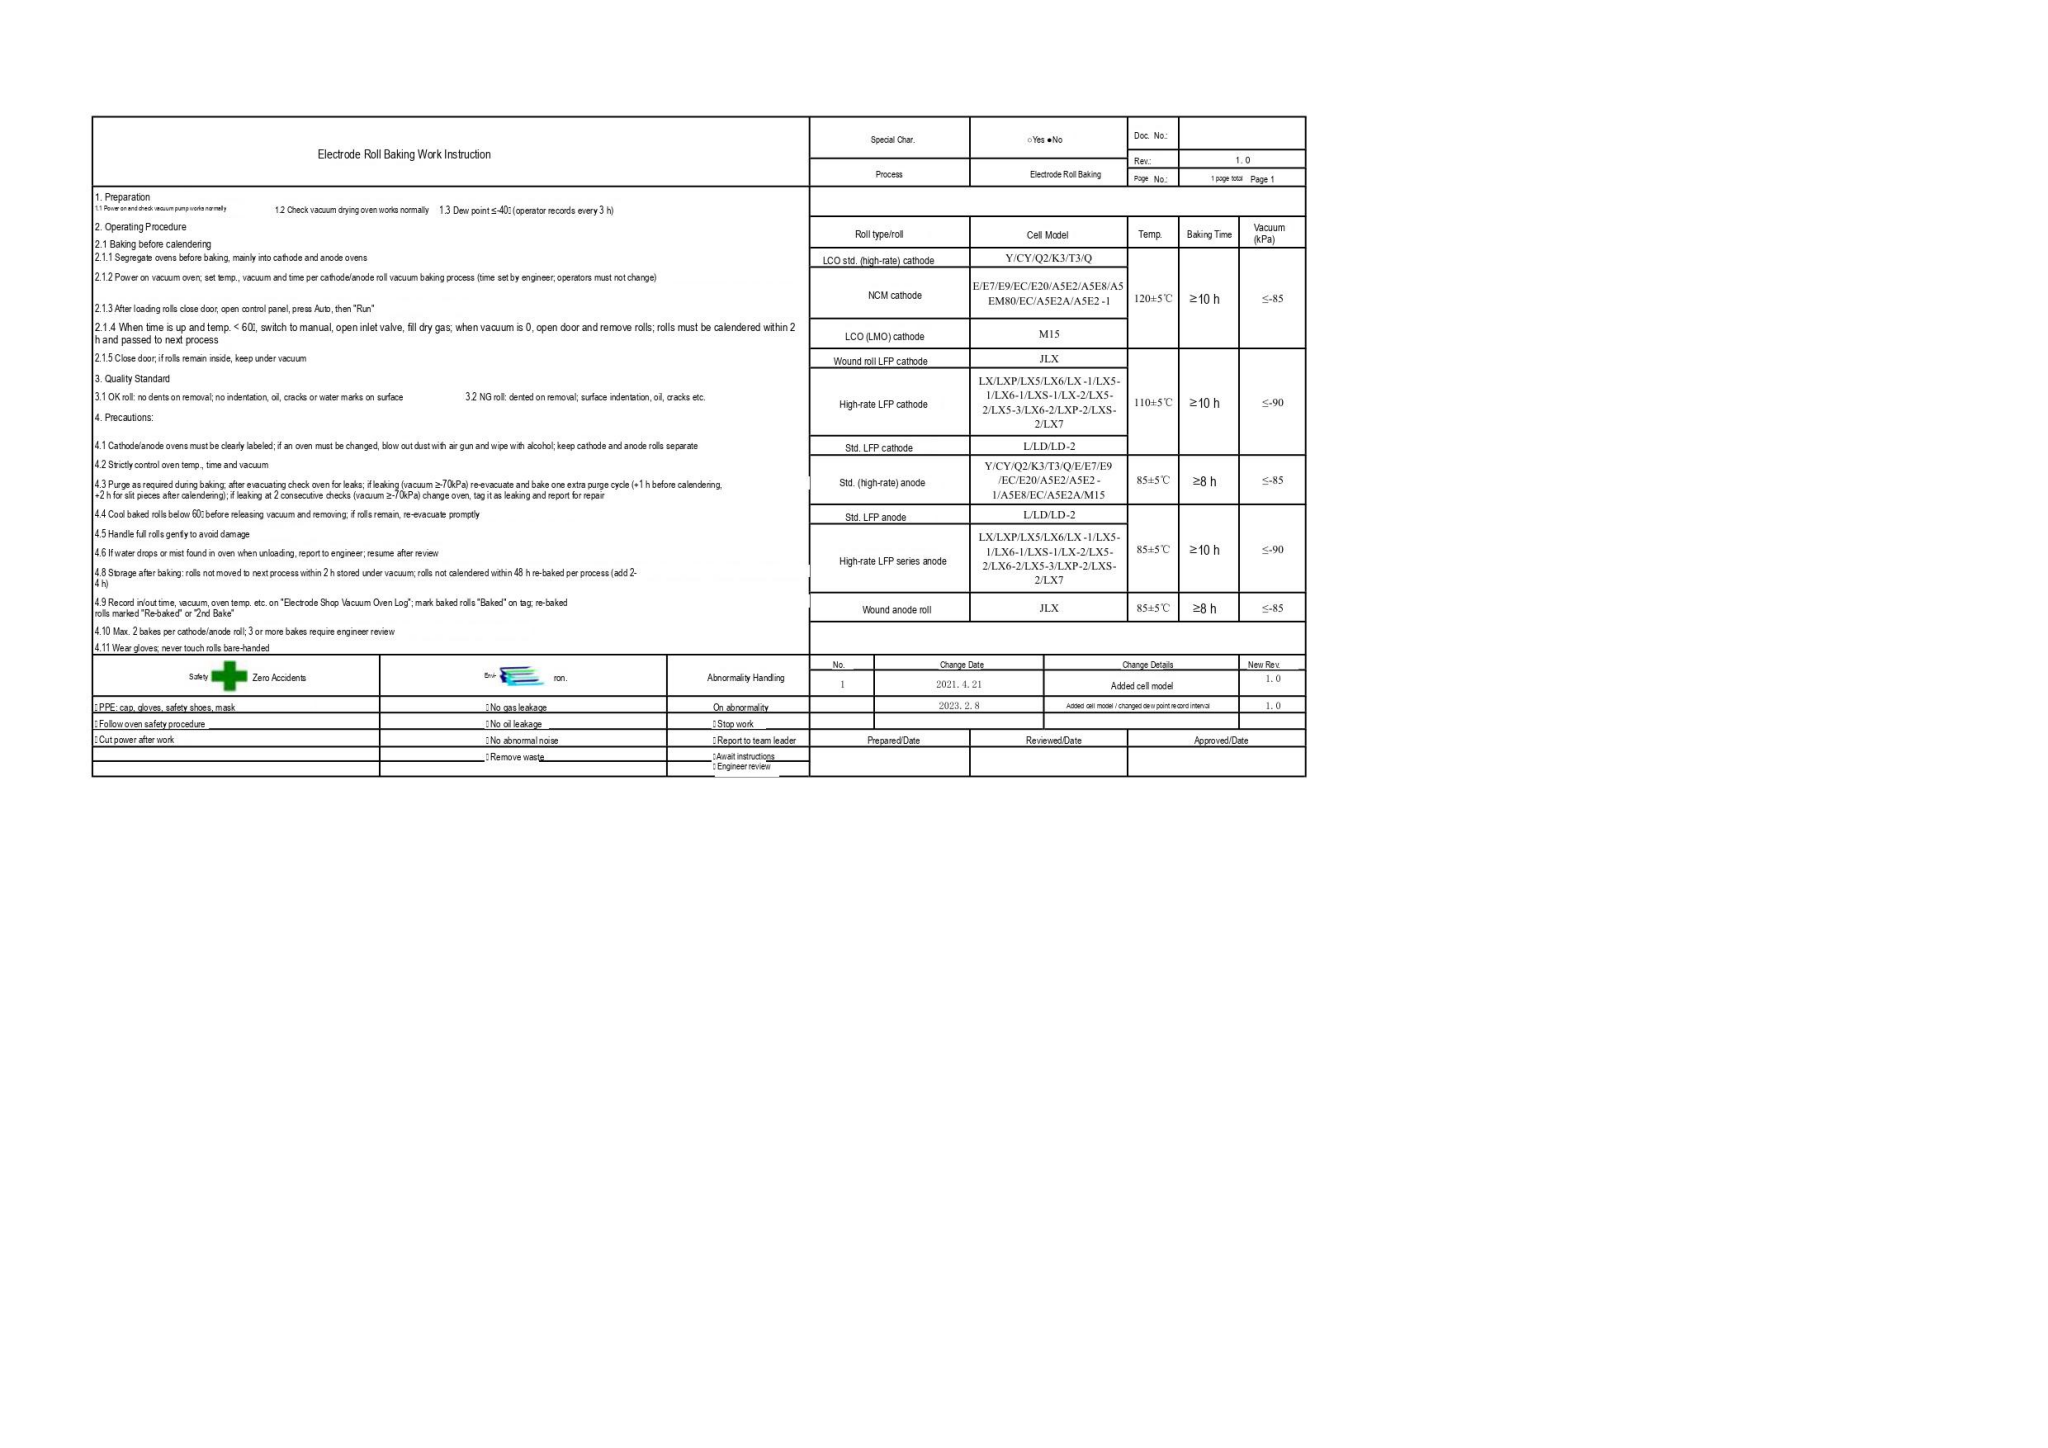| Electrode Roll Baking Work Instruction | Special Char. | ○Yes ●No | Doc. No.: | |
|---|---|---|---|---|
| | Process | Electrode Roll Baking | Rev.: | 1.0 |
| | | | Page No.: | 1 page total Page 1 |

1. Preparation
1.1 Power on and check vacuum pump works normally 1.2 Check vacuum drying oven works normally 1.3 Dew point ≤-40 (operator records every 3 h)
2. Operating Procedure
2.1 Baking before calendering
2.1.1 Segregate ovens before baking, mainly into cathode and anode ovens
2.1.2 Power on vacuum oven; set temp., vacuum and time per cathode/anode roll vacuum baking process (time set by engineer; operators must not change)
2.1.3 After loading rolls close door, open control panel, press Auto, then "Run"
2.1.4 When time is up and temp. < 60, switch to manual, open inlet valve, fill dry gas; when vacuum is 0, open door and remove rolls; rolls must be calendered within 2 h and passed to next process
2.1.5 Close door; if rolls remain inside, keep under vacuum
3. Quality Standard
3.1 OK roll: no dents on removal; no indentation, oil, cracks or water marks on surface 3.2 NG roll: dented on removal; surface indentation, oil, cracks etc.
4. Precautions:
4.1 Cathode/anode ovens must be clearly labeled; if an oven must be changed, blow out dust with air gun and wipe with alcohol; keep cathode and anode rolls separate
4.2 Strictly control oven temp., time and vacuum
4.3 Purge as required during baking; after evacuating check oven for leaks; if leaking (vacuum ≥-70kPa) re-evacuate and bake one extra purge cycle (+1 h before calendering, +2 h for slit pieces after calendering); if leaking at 2 consecutive checks (vacuum ≥-70kPa) change oven, tag it as leaking and report for repair
4.4 Cool baked rolls below 60 before releasing vacuum and removing; if rolls remain, re-evacuate promptly
4.5 Handle full rolls gently to avoid damage
4.6 If water drops or mist found in oven when unloading, report to engineer; resume after review
4.8 Storage after baking: rolls not moved to next process within 2 h stored under vacuum; rolls not calendered within 48 h re-baked per process (add 2-4 h)
4.9 Record in/out time, vacuum, oven temp. etc. on "Electrode Shop Vacuum Oven Log"; mark baked rolls "Baked" on tag; re-baked rolls marked "Re-baked" or "2nd Bake"
4.10 Max. 2 bakes per cathode/anode roll; 3 or more bakes require engineer review
4.11 Wear gloves; never touch rolls bare-handed

| Roll type/roll | Cell Model | Temp. | Baking Time | Vacuum (kPa) |
|---|---|---|---|---|
| LCO std. (high-rate) cathode | Y/CY/Q2/K3/T3/Q | | | |
| NCM cathode | E/E7/E9/EC/E20/A5E2/A5E8/A5EM80/EC/A5E2A/A5E2 -1 | 120±5℃ | ≥10 h | ≤-85 |
| LCO (LMO) cathode | M15 | | | |
| Wound roll LFP cathode | JLX | | | |
| High-rate LFP cathode | LX/LXP/LX5/LX6/LX -1/LX5-1/LX6-1/LXS-1/LX-2/LX5-2/LX5-3/LX6-2/LXP-2/LXS-2/LX7 | 110±5℃ | ≥10 h | ≤-90 |
| Std. LFP cathode | L/LD/LD-2 | | | |
| Std. (high-rate) anode | Y/CY/Q2/K3/T3/Q/E/E7/E9/EC/E20/A5E2/A5E2 -1/A5E8/EC/A5E2A/M15 | 85±5℃ | ≥8 h | ≤-85 |
| Std. LFP anode | L/LD/LD-2 | | | |
| High-rate LFP series anode | LX/LXP/LX5/LX6/LX -1/LX5-1/LX6-1/LXS-1/LX-2/LX5-2/LX6-2/LX5-3/LXP-2/LXS-2/LX7 | 85±5℃ | ≥10 h | ≤-90 |
| Wound anode roll | JLX | 85±5℃ | ≥8 h | ≤-85 |

| Safety Zero Accidents | Envir ron. | Abnormality Handling |
|---|---|---|
| PPE: cap, gloves, safety shoes, mask | No gas leakage | On abnormality |
| Follow oven safety procedure | No oil leakage | Stop work |
| Cut power after work | No abnormal noise | Report to team leader |
| | Remove waste | Await instructions<br>Engineer review |

| No. | Change Date | Change Details | New Rev. |
|---|---|---|---|
| 1 | 2021. 4. 21 | Added cell model | 1.0 |
| | 2023. 2. 8 | Added cell model / changed dew point record interval | 1.0 |

| Prepared/Date | Reviewed/Date | Approved/Date |
|---|---|---|
| | | |